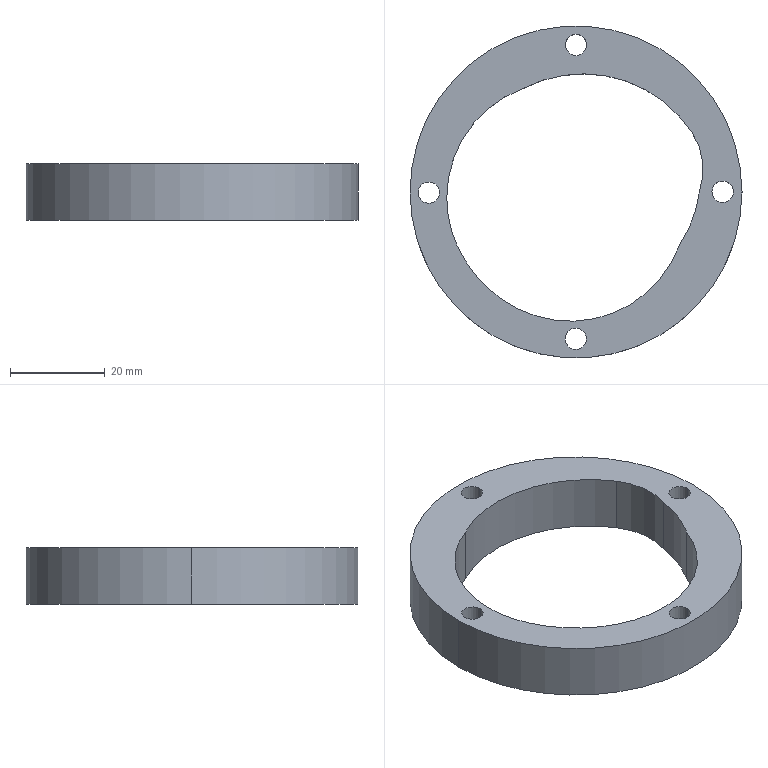Part | SolidWorks | features Extrusion 1, ICE 1 | 1 solid | 19 faces | box 70 x 70 x 12 mm | volume 19285 mm3 | cylinder 17 | plane 2 | commonest cylinder face diameters 4.5 x8 49 x3 55 x2 70 x2 28.257 x1 50.6 x1
STEP:
#1=CARTESIAN_POINT('',(28.668,0.04939,0.));
#2=VERTEX_POINT('',#1);
#3=CARTESIAN_POINT('',(33.168,0.04939,0.));
#4=VERTEX_POINT('',#3);
#5=CARTESIAN_POINT('',(30.918,0.04939,0.));
#6=DIRECTION('',(0.,0.,1.));
#7=DIRECTION('',(1.,0.,0.));
#8=AXIS2_PLACEMENT_3D('',#5,#6,#7);
#9=CIRCLE('',#8,2.25);
#10=EDGE_CURVE('',#2,#4,#9,.T.);
#11=ORIENTED_EDGE('',*,*,#10,.F.);
#12=CARTESIAN_POINT('',(28.668,0.04939,12.));
#13=VERTEX_POINT('',#12);
#14=CARTESIAN_POINT('',(28.668,0.04939,0.));
#15=DIRECTION('',(0.,0.,1.));
#16=VECTOR('',#15,1000.);
#17=LINE('',#14,#16);
#18=EDGE_CURVE('',#2,#13,#17,.T.);
#19=ORIENTED_EDGE('',*,*,#18,.T.);
#20=CARTESIAN_POINT('',(33.168,0.04939,12.));
#21=VERTEX_POINT('',#20);
#22=CARTESIAN_POINT('',(30.918,0.04939,12.));
#23=DIRECTION('',(0.,0.,1.));
#24=DIRECTION('',(1.,0.,0.));
#25=AXIS2_PLACEMENT_3D('',#22,#23,#24);
#26=CIRCLE('',#25,2.25);
#27=EDGE_CURVE('',#13,#21,#26,.T.);
#28=ORIENTED_EDGE('',*,*,#27,.T.);
#29=CARTESIAN_POINT('',(33.168,0.04939,0.));
#30=DIRECTION('',(0.,0.,1.));
#31=VECTOR('',#30,1000.);
#32=LINE('',#29,#31);
#33=EDGE_CURVE('',#4,#21,#32,.T.);
#34=ORIENTED_EDGE('',*,*,#33,.F.);
#35=EDGE_LOOP('',(#11,#19,#28,#34));
#36=FACE_OUTER_BOUND('',#35,.T.);
#37=CARTESIAN_POINT('',(30.918,0.04939,0.));
#38=DIRECTION('',(0.,0.,1.));
#39=DIRECTION('',(1.,0.,0.));
#40=AXIS2_PLACEMENT_3D('',#37,#38,#39);
#41=CYLINDRICAL_SURFACE('',#40,2.25);
#42=ADVANCED_FACE('',(#36),#41,.F.);
#43=CARTESIAN_POINT('',(-2.297,-30.979,0.));
#44=VERTEX_POINT('',#43);
#45=CARTESIAN_POINT('',(2.203,-30.979,0.));
#46=VERTEX_POINT('',#45);
#47=CARTESIAN_POINT('',(-0.04741,-30.979,0.));
#48=DIRECTION('',(0.,0.,1.));
#49=DIRECTION('',(1.,0.,0.));
#50=AXIS2_PLACEMENT_3D('',#47,#48,#49);
#51=CIRCLE('',#50,2.25);
#52=EDGE_CURVE('',#44,#46,#51,.T.);
#53=ORIENTED_EDGE('',*,*,#52,.F.);
#54=CARTESIAN_POINT('',(-2.297,-30.979,12.));
#55=VERTEX_POINT('',#54);
#56=CARTESIAN_POINT('',(-2.297,-30.979,0.));
#57=DIRECTION('',(0.,0.,1.));
#58=VECTOR('',#57,1000.);
#59=LINE('',#56,#58);
#60=EDGE_CURVE('',#44,#55,#59,.T.);
#61=ORIENTED_EDGE('',*,*,#60,.T.);
#62=CARTESIAN_POINT('',(2.203,-30.979,12.));
#63=VERTEX_POINT('',#62);
#64=CARTESIAN_POINT('',(-0.04741,-30.979,12.));
#65=DIRECTION('',(0.,0.,1.));
#66=DIRECTION('',(1.,0.,0.));
#67=AXIS2_PLACEMENT_3D('',#64,#65,#66);
#68=CIRCLE('',#67,2.25);
#69=EDGE_CURVE('',#55,#63,#68,.T.);
#70=ORIENTED_EDGE('',*,*,#69,.T.);
#71=CARTESIAN_POINT('',(2.203,-30.979,0.));
#72=DIRECTION('',(0.,0.,1.));
#73=VECTOR('',#72,1000.);
#74=LINE('',#71,#73);
#75=EDGE_CURVE('',#46,#63,#74,.T.);
#76=ORIENTED_EDGE('',*,*,#75,.F.);
#77=EDGE_LOOP('',(#53,#61,#70,#76));
#78=FACE_OUTER_BOUND('',#77,.T.);
#79=CARTESIAN_POINT('',(-0.04741,-30.979,0.));
#80=DIRECTION('',(0.,0.,1.));
#81=DIRECTION('',(1.,0.,0.));
#82=AXIS2_PLACEMENT_3D('',#79,#80,#81);
#83=CYLINDRICAL_SURFACE('',#82,2.25);
#84=ADVANCED_FACE('',(#78),#83,.F.);
#85=CARTESIAN_POINT('',(-33.267,-0.1482,0.));
#86=VERTEX_POINT('',#85);
#87=CARTESIAN_POINT('',(-28.767,-0.1482,0.));
#88=VERTEX_POINT('',#87);
#89=CARTESIAN_POINT('',(-31.017,-0.1482,0.));
#90=DIRECTION('',(0.,0.,1.));
#91=DIRECTION('',(1.,0.,0.));
#92=AXIS2_PLACEMENT_3D('',#89,#90,#91);
#93=CIRCLE('',#92,2.25);
#94=EDGE_CURVE('',#86,#88,#93,.T.);
#95=ORIENTED_EDGE('',*,*,#94,.F.);
#96=CARTESIAN_POINT('',(-33.267,-0.1482,12.));
#97=VERTEX_POINT('',#96);
#98=CARTESIAN_POINT('',(-33.267,-0.1482,0.));
#99=DIRECTION('',(0.,0.,1.));
#100=VECTOR('',#99,1000.);
#101=LINE('',#98,#100);
#102=EDGE_CURVE('',#86,#97,#101,.T.);
#103=ORIENTED_EDGE('',*,*,#102,.T.);
#104=CARTESIAN_POINT('',(-28.767,-0.1482,12.));
#105=VERTEX_POINT('',#104);
#106=CARTESIAN_POINT('',(-31.017,-0.1482,12.));
#107=DIRECTION('',(0.,0.,1.));
#108=DIRECTION('',(1.,0.,0.));
#109=AXIS2_PLACEMENT_3D('',#106,#107,#108);
#110=CIRCLE('',#109,2.25);
#111=EDGE_CURVE('',#97,#105,#110,.T.);
#112=ORIENTED_EDGE('',*,*,#111,.T.);
#113=CARTESIAN_POINT('',(-28.767,-0.1482,0.));
#114=DIRECTION('',(0.,0.,1.));
#115=VECTOR('',#114,1000.);
#116=LINE('',#113,#115);
#117=EDGE_CURVE('',#88,#105,#116,.T.);
#118=ORIENTED_EDGE('',*,*,#117,.F.);
#119=EDGE_LOOP('',(#95,#103,#112,#118));
#120=FACE_OUTER_BOUND('',#119,.T.);
#121=CARTESIAN_POINT('',(-31.017,-0.1482,0.));
#122=DIRECTION('',(0.,0.,1.));
#123=DIRECTION('',(1.,0.,0.));
#124=AXIS2_PLACEMENT_3D('',#121,#122,#123);
#125=CYLINDRICAL_SURFACE('',#124,2.25);
#126=ADVANCED_FACE('',(#120),#125,.F.);
#127=CARTESIAN_POINT('',(-2.25,31.,0.));
#128=VERTEX_POINT('',#127);
#129=CARTESIAN_POINT('',(2.25,31.,0.));
#130=VERTEX_POINT('',#129);
#131=CARTESIAN_POINT('',(0.,31.,0.));
#132=DIRECTION('',(0.,0.,1.));
#133=DIRECTION('',(1.,0.,0.));
#134=AXIS2_PLACEMENT_3D('',#131,#132,#133);
#135=CIRCLE('',#134,2.25);
#136=EDGE_CURVE('',#128,#130,#135,.T.);
#137=ORIENTED_EDGE('',*,*,#136,.F.);
#138=CARTESIAN_POINT('',(-2.25,31.,12.));
#139=VERTEX_POINT('',#138);
#140=CARTESIAN_POINT('',(-2.25,31.,0.));
#141=DIRECTION('',(0.,0.,1.));
#142=VECTOR('',#141,1000.);
#143=LINE('',#140,#142);
#144=EDGE_CURVE('',#128,#139,#143,.T.);
#145=ORIENTED_EDGE('',*,*,#144,.T.);
#146=CARTESIAN_POINT('',(2.25,31.,12.));
#147=VERTEX_POINT('',#146);
#148=CARTESIAN_POINT('',(0.,31.,12.));
#149=DIRECTION('',(0.,0.,1.));
#150=DIRECTION('',(1.,0.,0.));
#151=AXIS2_PLACEMENT_3D('',#148,#149,#150);
#152=CIRCLE('',#151,2.25);
#153=EDGE_CURVE('',#139,#147,#152,.T.);
#154=ORIENTED_EDGE('',*,*,#153,.T.);
#155=CARTESIAN_POINT('',(2.25,31.,0.));
#156=DIRECTION('',(0.,0.,1.));
#157=VECTOR('',#156,1000.);
#158=LINE('',#155,#157);
#159=EDGE_CURVE('',#130,#147,#158,.T.);
#160=ORIENTED_EDGE('',*,*,#159,.F.);
#161=EDGE_LOOP('',(#137,#145,#154,#160));
#162=FACE_OUTER_BOUND('',#161,.T.);
#163=CARTESIAN_POINT('',(0.,31.,0.));
#164=DIRECTION('',(0.,0.,1.));
#165=DIRECTION('',(1.,0.,0.));
#166=AXIS2_PLACEMENT_3D('',#163,#164,#165);
#167=CYLINDRICAL_SURFACE('',#166,2.25);
#168=ADVANCED_FACE('',(#162),#167,.F.);
#169=CARTESIAN_POINT('',(35.,0.,12.));
#170=VERTEX_POINT('',#169);
#171=CARTESIAN_POINT('',(-35.,0.,12.));
#172=VERTEX_POINT('',#171);
#173=CARTESIAN_POINT('',(0.,0.,12.));
#174=DIRECTION('',(0.,0.,1.));
#175=DIRECTION('',(1.,0.,0.));
#176=AXIS2_PLACEMENT_3D('',#173,#174,#175);
#177=CIRCLE('',#176,35.);
#178=EDGE_CURVE('',#170,#172,#177,.T.);
#179=ORIENTED_EDGE('',*,*,#178,.F.);
#180=CARTESIAN_POINT('',(35.,0.,0.));
#181=VERTEX_POINT('',#180);
#182=CARTESIAN_POINT('',(35.,0.,12.));
#183=DIRECTION('',(0.,0.,-1.));
#184=VECTOR('',#183,1000.);
#185=LINE('',#182,#184);
#186=EDGE_CURVE('',#170,#181,#185,.T.);
#187=ORIENTED_EDGE('',*,*,#186,.T.);
#188=CARTESIAN_POINT('',(-35.,0.,0.));
#189=VERTEX_POINT('',#188);
#190=CARTESIAN_POINT('',(0.,0.,0.));
#191=DIRECTION('',(0.,0.,1.));
#192=DIRECTION('',(1.,0.,0.));
#193=AXIS2_PLACEMENT_3D('',#190,#191,#192);
#194=CIRCLE('',#193,35.);
#195=EDGE_CURVE('',#181,#189,#194,.T.);
#196=ORIENTED_EDGE('',*,*,#195,.T.);
#197=CARTESIAN_POINT('',(-35.,0.,12.));
#198=DIRECTION('',(0.,0.,-1.));
#199=VECTOR('',#198,1000.);
#200=LINE('',#197,#199);
#201=EDGE_CURVE('',#172,#189,#200,.T.);
#202=ORIENTED_EDGE('',*,*,#201,.F.);
#203=EDGE_LOOP('',(#179,#187,#196,#202));
#204=FACE_OUTER_BOUND('',#203,.T.);
#205=CARTESIAN_POINT('',(0.,0.,12.));
#206=DIRECTION('',(0.,0.,-1.));
#207=DIRECTION('',(-1.,0.,0.));
#208=AXIS2_PLACEMENT_3D('',#205,#206,#207);
#209=CYLINDRICAL_SURFACE('',#208,35.);
#210=ADVANCED_FACE('',(#204),#209,.T.);
#211=CARTESIAN_POINT('',(-27.251,-1.196,12.));
#212=VERTEX_POINT('',#211);
#213=CARTESIAN_POINT('',(-11.123,21.83,12.));
#214=VERTEX_POINT('',#213);
#215=CARTESIAN_POINT('',(-2.751,-1.196,12.));
#216=DIRECTION('',(0.,0.,-1.));
#217=DIRECTION('',(1.,0.,0.));
#218=AXIS2_PLACEMENT_3D('',#215,#216,#217);
#219=CIRCLE('',#218,24.5);
#220=EDGE_CURVE('',#212,#214,#219,.T.);
#221=ORIENTED_EDGE('',*,*,#220,.F.);
#222=CARTESIAN_POINT('',(-27.251,-1.196,0.));
#223=VERTEX_POINT('',#222);
#224=CARTESIAN_POINT('',(-27.251,-1.196,12.));
#225=DIRECTION('',(0.,0.,-1.));
#226=VECTOR('',#225,1000.);
#227=LINE('',#224,#226);
#228=EDGE_CURVE('',#212,#223,#227,.T.);
#229=ORIENTED_EDGE('',*,*,#228,.T.);
#230=CARTESIAN_POINT('',(-11.123,21.83,0.));
#231=VERTEX_POINT('',#230);
#232=CARTESIAN_POINT('',(-2.751,-1.196,0.));
#233=DIRECTION('',(0.,0.,-1.));
#234=DIRECTION('',(1.,0.,0.));
#235=AXIS2_PLACEMENT_3D('',#232,#233,#234);
#236=CIRCLE('',#235,24.5);
#237=EDGE_CURVE('',#223,#231,#236,.T.);
#238=ORIENTED_EDGE('',*,*,#237,.T.);
#239=CARTESIAN_POINT('',(-11.123,21.83,12.));
#240=DIRECTION('',(0.,0.,-1.));
#241=VECTOR('',#240,1000.);
#242=LINE('',#239,#241);
#243=EDGE_CURVE('',#214,#231,#242,.T.);
#244=ORIENTED_EDGE('',*,*,#243,.F.);
#245=EDGE_LOOP('',(#221,#229,#238,#244));
#246=FACE_OUTER_BOUND('',#245,.T.);
#247=CARTESIAN_POINT('',(-2.751,-1.196,12.));
#248=DIRECTION('',(0.,0.,-1.));
#249=DIRECTION('',(-1.,0.,0.));
#250=AXIS2_PLACEMENT_3D('',#247,#248,#249);
#251=CYLINDRICAL_SURFACE('',#250,24.5);
#252=ADVANCED_FACE('',(#246),#251,.F.);
#253=CARTESIAN_POINT('',(-12.485,-24.503,0.));
#254=VERTEX_POINT('',#253);
#255=CARTESIAN_POINT('',(21.83,-11.123,0.));
#256=VERTEX_POINT('',#255);
#257=CARTESIAN_POINT('',(-1.198,-2.757,0.));
#258=DIRECTION('',(0.,0.,1.));
#259=DIRECTION('',(1.,0.,0.));
#260=AXIS2_PLACEMENT_3D('',#257,#258,#259);
#261=CIRCLE('',#260,24.5);
#262=EDGE_CURVE('',#254,#256,#261,.T.);
#263=ORIENTED_EDGE('',*,*,#262,.F.);
#264=CARTESIAN_POINT('',(-12.485,-24.503,12.));
#265=VERTEX_POINT('',#264);
#266=CARTESIAN_POINT('',(-12.485,-24.503,12.));
#267=DIRECTION('',(0.,0.,-1.));
#268=VECTOR('',#267,1000.);
#269=LINE('',#266,#268);
#270=EDGE_CURVE('',#265,#254,#269,.T.);
#271=ORIENTED_EDGE('',*,*,#270,.F.);
#272=CARTESIAN_POINT('',(21.83,-11.123,12.));
#273=VERTEX_POINT('',#272);
#274=CARTESIAN_POINT('',(-1.198,-2.757,12.));
#275=DIRECTION('',(0.,0.,1.));
#276=DIRECTION('',(1.,0.,0.));
#277=AXIS2_PLACEMENT_3D('',#274,#275,#276);
#278=CIRCLE('',#277,24.5);
#279=EDGE_CURVE('',#265,#273,#278,.T.);
#280=ORIENTED_EDGE('',*,*,#279,.T.);
#281=CARTESIAN_POINT('',(21.83,-11.123,12.));
#282=DIRECTION('',(0.,0.,-1.));
#283=VECTOR('',#282,1000.);
#284=LINE('',#281,#283);
#285=EDGE_CURVE('',#273,#256,#284,.T.);
#286=ORIENTED_EDGE('',*,*,#285,.T.);
#287=EDGE_LOOP('',(#263,#271,#280,#286));
#288=FACE_OUTER_BOUND('',#287,.T.);
#289=CARTESIAN_POINT('',(-1.198,-2.757,12.));
#290=DIRECTION('',(0.,0.,-1.));
#291=DIRECTION('',(-1.,0.,0.));
#292=AXIS2_PLACEMENT_3D('',#289,#290,#291);
#293=CYLINDRICAL_SURFACE('',#292,24.5);
#294=ADVANCED_FACE('',(#288),#293,.F.);
#295=CARTESIAN_POINT('',(-25.221,-10.961,0.));
#296=VERTEX_POINT('',#295);
#297=CARTESIAN_POINT('',(0.,0.,0.));
#298=DIRECTION('',(0.,0.,1.));
#299=DIRECTION('',(1.,0.,0.));
#300=AXIS2_PLACEMENT_3D('',#297,#298,#299);
#301=CIRCLE('',#300,27.5);
#302=EDGE_CURVE('',#296,#254,#301,.T.);
#303=ORIENTED_EDGE('',*,*,#302,.F.);
#304=CARTESIAN_POINT('',(-25.221,-10.961,12.));
#305=VERTEX_POINT('',#304);
#306=CARTESIAN_POINT('',(-25.221,-10.961,12.));
#307=DIRECTION('',(0.,0.,-1.));
#308=VECTOR('',#307,1000.);
#309=LINE('',#306,#308);
#310=EDGE_CURVE('',#305,#296,#309,.T.);
#311=ORIENTED_EDGE('',*,*,#310,.F.);
#312=CARTESIAN_POINT('',(0.,0.,12.));
#313=DIRECTION('',(0.,0.,1.));
#314=DIRECTION('',(1.,0.,0.));
#315=AXIS2_PLACEMENT_3D('',#312,#313,#314);
#316=CIRCLE('',#315,27.5);
#317=EDGE_CURVE('',#305,#265,#316,.T.);
#318=ORIENTED_EDGE('',*,*,#317,.T.);
#319=ORIENTED_EDGE('',*,*,#270,.T.);
#320=EDGE_LOOP('',(#303,#311,#318,#319));
#321=FACE_OUTER_BOUND('',#320,.T.);
#322=CARTESIAN_POINT('',(0.,0.,12.));
#323=DIRECTION('',(0.,0.,-1.));
#324=DIRECTION('',(-1.,0.,0.));
#325=AXIS2_PLACEMENT_3D('',#322,#323,#324);
#326=CYLINDRICAL_SURFACE('',#325,27.5);
#327=ADVANCED_FACE('',(#321),#326,.F.);
#328=ORIENTED_EDGE('',*,*,#228,.F.);
#329=CARTESIAN_POINT('',(-2.751,-1.196,12.));
#330=DIRECTION('',(0.,0.,-1.));
#331=DIRECTION('',(1.,0.,0.));
#332=AXIS2_PLACEMENT_3D('',#329,#330,#331);
#333=CIRCLE('',#332,24.5);
#334=EDGE_CURVE('',#305,#212,#333,.T.);
#335=ORIENTED_EDGE('',*,*,#334,.F.);
#336=ORIENTED_EDGE('',*,*,#310,.T.);
#337=CARTESIAN_POINT('',(-2.751,-1.196,0.));
#338=DIRECTION('',(0.,0.,-1.));
#339=DIRECTION('',(1.,0.,0.));
#340=AXIS2_PLACEMENT_3D('',#337,#338,#339);
#341=CIRCLE('',#340,24.5);
#342=EDGE_CURVE('',#296,#223,#341,.T.);
#343=ORIENTED_EDGE('',*,*,#342,.T.);
#344=EDGE_LOOP('',(#328,#335,#336,#343));
#345=FACE_OUTER_BOUND('',#344,.T.);
#346=CARTESIAN_POINT('',(-2.751,-1.196,12.));
#347=DIRECTION('',(0.,0.,-1.));
#348=DIRECTION('',(-1.,0.,0.));
#349=AXIS2_PLACEMENT_3D('',#346,#347,#348);
#350=CYLINDRICAL_SURFACE('',#349,24.5);
#351=ADVANCED_FACE('',(#345),#350,.F.);
#352=CARTESIAN_POINT('',(24.503,12.485,0.));
#353=VERTEX_POINT('',#352);
#354=CARTESIAN_POINT('',(1.508,-2.598,0.));
#355=DIRECTION('',(0.,0.,-1.));
#356=DIRECTION('',(1.,0.,0.));
#357=AXIS2_PLACEMENT_3D('',#354,#355,#356);
#358=CIRCLE('',#357,27.5);
#359=EDGE_CURVE('',#231,#353,#358,.T.);
#360=ORIENTED_EDGE('',*,*,#359,.T.);
#361=CARTESIAN_POINT('',(24.503,12.485,12.));
#362=VERTEX_POINT('',#361);
#363=CARTESIAN_POINT('',(24.503,12.485,12.));
#364=DIRECTION('',(0.,0.,-1.));
#365=VECTOR('',#364,1000.);
#366=LINE('',#363,#365);
#367=EDGE_CURVE('',#362,#353,#366,.T.);
#368=ORIENTED_EDGE('',*,*,#367,.F.);
#369=CARTESIAN_POINT('',(1.508,-2.598,12.));
#370=DIRECTION('',(0.,0.,-1.));
#371=DIRECTION('',(1.,0.,0.));
#372=AXIS2_PLACEMENT_3D('',#369,#370,#371);
#373=CIRCLE('',#372,27.5);
#374=EDGE_CURVE('',#214,#362,#373,.T.);
#375=ORIENTED_EDGE('',*,*,#374,.F.);
#376=ORIENTED_EDGE('',*,*,#243,.T.);
#377=EDGE_LOOP('',(#360,#368,#375,#376));
#378=FACE_OUTER_BOUND('',#377,.T.);
#379=CARTESIAN_POINT('',(1.508,-2.598,12.));
#380=DIRECTION('',(0.,0.,-1.));
#381=DIRECTION('',(-1.,0.,0.));
#382=AXIS2_PLACEMENT_3D('',#379,#380,#381);
#383=CYLINDRICAL_SURFACE('',#382,27.5);
#384=ADVANCED_FACE('',(#378),#383,.F.);
#385=CARTESIAN_POINT('',(26.,0.,0.));
#386=VERTEX_POINT('',#385);
#387=CARTESIAN_POINT('',(12.689,4.736,0.));
#388=DIRECTION('',(0.,0.,-1.));
#389=DIRECTION('',(1.,0.,0.));
#390=AXIS2_PLACEMENT_3D('',#387,#388,#389);
#391=CIRCLE('',#390,14.129);
#392=EDGE_CURVE('',#353,#386,#391,.T.);
#393=ORIENTED_EDGE('',*,*,#392,.T.);
#394=CARTESIAN_POINT('',(26.,0.,12.));
#395=VERTEX_POINT('',#394);
#396=CARTESIAN_POINT('',(26.,0.,12.));
#397=DIRECTION('',(0.,0.,-1.));
#398=VECTOR('',#397,1000.);
#399=LINE('',#396,#398);
#400=EDGE_CURVE('',#395,#386,#399,.T.);
#401=ORIENTED_EDGE('',*,*,#400,.F.);
#402=CARTESIAN_POINT('',(12.689,4.736,12.));
#403=DIRECTION('',(0.,0.,-1.));
#404=DIRECTION('',(1.,0.,0.));
#405=AXIS2_PLACEMENT_3D('',#402,#403,#404);
#406=CIRCLE('',#405,14.129);
#407=EDGE_CURVE('',#362,#395,#406,.T.);
#408=ORIENTED_EDGE('',*,*,#407,.F.);
#409=ORIENTED_EDGE('',*,*,#367,.T.);
#410=EDGE_LOOP('',(#393,#401,#408,#409));
#411=FACE_OUTER_BOUND('',#410,.T.);
#412=CARTESIAN_POINT('',(12.689,4.736,12.));
#413=DIRECTION('',(0.,0.,-1.));
#414=DIRECTION('',(-1.,0.,0.));
#415=AXIS2_PLACEMENT_3D('',#412,#413,#414);
#416=CYLINDRICAL_SURFACE('',#415,14.129);
#417=ADVANCED_FACE('',(#411),#416,.F.);
#418=CARTESIAN_POINT('',(0.8873,3.073,0.));
#419=DIRECTION('',(0.,0.,-1.));
#420=DIRECTION('',(1.,0.,0.));
#421=AXIS2_PLACEMENT_3D('',#418,#419,#420);
#422=CIRCLE('',#421,25.3);
#423=EDGE_CURVE('',#386,#256,#422,.T.);
#424=ORIENTED_EDGE('',*,*,#423,.T.);
#425=ORIENTED_EDGE('',*,*,#285,.F.);
#426=CARTESIAN_POINT('',(0.8873,3.073,12.));
#427=DIRECTION('',(0.,0.,-1.));
#428=DIRECTION('',(1.,0.,0.));
#429=AXIS2_PLACEMENT_3D('',#426,#427,#428);
#430=CIRCLE('',#429,25.3);
#431=EDGE_CURVE('',#395,#273,#430,.T.);
#432=ORIENTED_EDGE('',*,*,#431,.F.);
#433=ORIENTED_EDGE('',*,*,#400,.T.);
#434=EDGE_LOOP('',(#424,#425,#432,#433));
#435=FACE_OUTER_BOUND('',#434,.T.);
#436=CARTESIAN_POINT('',(0.8873,3.073,12.));
#437=DIRECTION('',(0.,0.,-1.));
#438=DIRECTION('',(-1.,0.,0.));
#439=AXIS2_PLACEMENT_3D('',#436,#437,#438);
#440=CYLINDRICAL_SURFACE('',#439,25.3);
#441=ADVANCED_FACE('',(#435),#440,.F.);
#442=ORIENTED_EDGE('',*,*,#186,.F.);
#443=CARTESIAN_POINT('',(0.,0.,12.));
#444=DIRECTION('',(0.,0.,1.));
#445=DIRECTION('',(1.,0.,0.));
#446=AXIS2_PLACEMENT_3D('',#443,#444,#445);
#447=CIRCLE('',#446,35.);
#448=EDGE_CURVE('',#172,#170,#447,.T.);
#449=ORIENTED_EDGE('',*,*,#448,.F.);
#450=ORIENTED_EDGE('',*,*,#201,.T.);
#451=CARTESIAN_POINT('',(0.,0.,0.));
#452=DIRECTION('',(0.,0.,1.));
#453=DIRECTION('',(1.,0.,0.));
#454=AXIS2_PLACEMENT_3D('',#451,#452,#453);
#455=CIRCLE('',#454,35.);
#456=EDGE_CURVE('',#189,#181,#455,.T.);
#457=ORIENTED_EDGE('',*,*,#456,.T.);
#458=EDGE_LOOP('',(#442,#449,#450,#457));
#459=FACE_OUTER_BOUND('',#458,.T.);
#460=CARTESIAN_POINT('',(0.,0.,12.));
#461=DIRECTION('',(0.,0.,-1.));
#462=DIRECTION('',(-1.,0.,0.));
#463=AXIS2_PLACEMENT_3D('',#460,#461,#462);
#464=CYLINDRICAL_SURFACE('',#463,35.);
#465=ADVANCED_FACE('',(#459),#464,.T.);
#466=CARTESIAN_POINT('',(30.918,0.04939,12.));
#467=DIRECTION('',(0.,0.,1.));
#468=DIRECTION('',(1.,0.,0.));
#469=AXIS2_PLACEMENT_3D('',#466,#467,#468);
#470=CIRCLE('',#469,2.25);
#471=EDGE_CURVE('',#21,#13,#470,.T.);
#472=ORIENTED_EDGE('',*,*,#471,.F.);
#473=ORIENTED_EDGE('',*,*,#27,.F.);
#474=EDGE_LOOP('',(#472,#473));
#475=FACE_BOUND('',#474,.T.);
#476=CARTESIAN_POINT('',(-0.04741,-30.979,12.));
#477=DIRECTION('',(0.,0.,1.));
#478=DIRECTION('',(1.,0.,0.));
#479=AXIS2_PLACEMENT_3D('',#476,#477,#478);
#480=CIRCLE('',#479,2.25);
#481=EDGE_CURVE('',#63,#55,#480,.T.);
#482=ORIENTED_EDGE('',*,*,#481,.F.);
#483=ORIENTED_EDGE('',*,*,#69,.F.);
#484=EDGE_LOOP('',(#482,#483));
#485=FACE_BOUND('',#484,.T.);
#486=CARTESIAN_POINT('',(-31.017,-0.1482,12.));
#487=DIRECTION('',(0.,0.,1.));
#488=DIRECTION('',(1.,0.,0.));
#489=AXIS2_PLACEMENT_3D('',#486,#487,#488);
#490=CIRCLE('',#489,2.25);
#491=EDGE_CURVE('',#105,#97,#490,.T.);
#492=ORIENTED_EDGE('',*,*,#491,.F.);
#493=ORIENTED_EDGE('',*,*,#111,.F.);
#494=EDGE_LOOP('',(#492,#493));
#495=FACE_BOUND('',#494,.T.);
#496=CARTESIAN_POINT('',(0.,31.,12.));
#497=DIRECTION('',(0.,0.,1.));
#498=DIRECTION('',(1.,0.,0.));
#499=AXIS2_PLACEMENT_3D('',#496,#497,#498);
#500=CIRCLE('',#499,2.25);
#501=EDGE_CURVE('',#147,#139,#500,.T.);
#502=ORIENTED_EDGE('',*,*,#501,.F.);
#503=ORIENTED_EDGE('',*,*,#153,.F.);
#504=EDGE_LOOP('',(#502,#503));
#505=FACE_BOUND('',#504,.T.);
#506=ORIENTED_EDGE('',*,*,#279,.F.);
#507=ORIENTED_EDGE('',*,*,#317,.F.);
#508=ORIENTED_EDGE('',*,*,#334,.T.);
#509=ORIENTED_EDGE('',*,*,#220,.T.);
#510=ORIENTED_EDGE('',*,*,#374,.T.);
#511=ORIENTED_EDGE('',*,*,#407,.T.);
#512=ORIENTED_EDGE('',*,*,#431,.T.);
#513=EDGE_LOOP('',(#506,#507,#508,#509,#510,#511,#512));
#514=FACE_BOUND('',#513,.T.);
#515=ORIENTED_EDGE('',*,*,#448,.T.);
#516=ORIENTED_EDGE('',*,*,#178,.T.);
#517=EDGE_LOOP('',(#515,#516));
#518=FACE_OUTER_BOUND('',#517,.T.);
#519=CARTESIAN_POINT('',(0.,0.,12.));
#520=DIRECTION('',(0.,0.,1.));
#521=DIRECTION('',(1.,0.,0.));
#522=AXIS2_PLACEMENT_3D('',#519,#520,#521);
#523=PLANE('',#522);
#524=ADVANCED_FACE('',(#475,#485,#495,#505,#514,#518),#523,.T.);
#525=CARTESIAN_POINT('',(30.918,0.04939,0.));
#526=DIRECTION('',(0.,0.,1.));
#527=DIRECTION('',(1.,0.,0.));
#528=AXIS2_PLACEMENT_3D('',#525,#526,#527);
#529=CIRCLE('',#528,2.25);
#530=EDGE_CURVE('',#4,#2,#529,.T.);
#531=ORIENTED_EDGE('',*,*,#530,.T.);
#532=ORIENTED_EDGE('',*,*,#10,.T.);
#533=EDGE_LOOP('',(#531,#532));
#534=FACE_BOUND('',#533,.T.);
#535=CARTESIAN_POINT('',(-0.04741,-30.979,0.));
#536=DIRECTION('',(0.,0.,1.));
#537=DIRECTION('',(1.,0.,0.));
#538=AXIS2_PLACEMENT_3D('',#535,#536,#537);
#539=CIRCLE('',#538,2.25);
#540=EDGE_CURVE('',#46,#44,#539,.T.);
#541=ORIENTED_EDGE('',*,*,#540,.T.);
#542=ORIENTED_EDGE('',*,*,#52,.T.);
#543=EDGE_LOOP('',(#541,#542));
#544=FACE_BOUND('',#543,.T.);
#545=CARTESIAN_POINT('',(-31.017,-0.1482,0.));
#546=DIRECTION('',(0.,0.,1.));
#547=DIRECTION('',(1.,0.,0.));
#548=AXIS2_PLACEMENT_3D('',#545,#546,#547);
#549=CIRCLE('',#548,2.25);
#550=EDGE_CURVE('',#88,#86,#549,.T.);
#551=ORIENTED_EDGE('',*,*,#550,.T.);
#552=ORIENTED_EDGE('',*,*,#94,.T.);
#553=EDGE_LOOP('',(#551,#552));
#554=FACE_BOUND('',#553,.T.);
#555=CARTESIAN_POINT('',(0.,31.,0.));
#556=DIRECTION('',(0.,0.,1.));
#557=DIRECTION('',(1.,0.,0.));
#558=AXIS2_PLACEMENT_3D('',#555,#556,#557);
#559=CIRCLE('',#558,2.25);
#560=EDGE_CURVE('',#130,#128,#559,.T.);
#561=ORIENTED_EDGE('',*,*,#560,.T.);
#562=ORIENTED_EDGE('',*,*,#136,.T.);
#563=EDGE_LOOP('',(#561,#562));
#564=FACE_BOUND('',#563,.T.);
#565=ORIENTED_EDGE('',*,*,#262,.T.);
#566=ORIENTED_EDGE('',*,*,#423,.F.);
#567=ORIENTED_EDGE('',*,*,#392,.F.);
#568=ORIENTED_EDGE('',*,*,#359,.F.);
#569=ORIENTED_EDGE('',*,*,#237,.F.);
#570=ORIENTED_EDGE('',*,*,#342,.F.);
#571=ORIENTED_EDGE('',*,*,#302,.T.);
#572=EDGE_LOOP('',(#565,#566,#567,#568,#569,#570,#571));
#573=FACE_BOUND('',#572,.T.);
#574=ORIENTED_EDGE('',*,*,#456,.F.);
#575=ORIENTED_EDGE('',*,*,#195,.F.);
#576=EDGE_LOOP('',(#574,#575));
#577=FACE_OUTER_BOUND('',#576,.T.);
#578=CARTESIAN_POINT('',(0.,0.,0.));
#579=DIRECTION('',(0.,0.,1.));
#580=DIRECTION('',(1.,0.,0.));
#581=AXIS2_PLACEMENT_3D('',#578,#579,#580);
#582=PLANE('',#581);
#583=ADVANCED_FACE('',(#534,#544,#554,#564,#573,#577),#582,.F.);
#584=ORIENTED_EDGE('',*,*,#144,.F.);
#585=ORIENTED_EDGE('',*,*,#560,.F.);
#586=ORIENTED_EDGE('',*,*,#159,.T.);
#587=ORIENTED_EDGE('',*,*,#501,.T.);
#588=EDGE_LOOP('',(#584,#585,#586,#587));
#589=FACE_OUTER_BOUND('',#588,.T.);
#590=CARTESIAN_POINT('',(0.,31.,0.));
#591=DIRECTION('',(0.,0.,1.));
#592=DIRECTION('',(1.,0.,0.));
#593=AXIS2_PLACEMENT_3D('',#590,#591,#592);
#594=CYLINDRICAL_SURFACE('',#593,2.25);
#595=ADVANCED_FACE('',(#589),#594,.F.);
#596=ORIENTED_EDGE('',*,*,#102,.F.);
#597=ORIENTED_EDGE('',*,*,#550,.F.);
#598=ORIENTED_EDGE('',*,*,#117,.T.);
#599=ORIENTED_EDGE('',*,*,#491,.T.);
#600=EDGE_LOOP('',(#596,#597,#598,#599));
#601=FACE_OUTER_BOUND('',#600,.T.);
#602=CARTESIAN_POINT('',(-31.017,-0.1482,0.));
#603=DIRECTION('',(0.,0.,1.));
#604=DIRECTION('',(1.,0.,0.));
#605=AXIS2_PLACEMENT_3D('',#602,#603,#604);
#606=CYLINDRICAL_SURFACE('',#605,2.25);
#607=ADVANCED_FACE('',(#601),#606,.F.);
#608=ORIENTED_EDGE('',*,*,#60,.F.);
#609=ORIENTED_EDGE('',*,*,#540,.F.);
#610=ORIENTED_EDGE('',*,*,#75,.T.);
#611=ORIENTED_EDGE('',*,*,#481,.T.);
#612=EDGE_LOOP('',(#608,#609,#610,#611));
#613=FACE_OUTER_BOUND('',#612,.T.);
#614=CARTESIAN_POINT('',(-0.04741,-30.979,0.));
#615=DIRECTION('',(0.,0.,1.));
#616=DIRECTION('',(1.,0.,0.));
#617=AXIS2_PLACEMENT_3D('',#614,#615,#616);
#618=CYLINDRICAL_SURFACE('',#617,2.25);
#619=ADVANCED_FACE('',(#613),#618,.F.);
#620=ORIENTED_EDGE('',*,*,#18,.F.);
#621=ORIENTED_EDGE('',*,*,#530,.F.);
#622=ORIENTED_EDGE('',*,*,#33,.T.);
#623=ORIENTED_EDGE('',*,*,#471,.T.);
#624=EDGE_LOOP('',(#620,#621,#622,#623));
#625=FACE_OUTER_BOUND('',#624,.T.);
#626=CARTESIAN_POINT('',(30.918,0.04939,0.));
#627=DIRECTION('',(0.,0.,1.));
#628=DIRECTION('',(1.,0.,0.));
#629=AXIS2_PLACEMENT_3D('',#626,#627,#628);
#630=CYLINDRICAL_SURFACE('',#629,2.25);
#631=ADVANCED_FACE('',(#625),#630,.F.);
#632=CLOSED_SHELL('',(#42,#84,#126,#168,#210,#252,#294,#327,#351,#384,#417,#441,#465,#524,#583,#595,#607,#619,#631));
#633=MANIFOLD_SOLID_BREP('',#632);
#634=CARTESIAN_POINT('',(0.,0.,0.));
#635=DIRECTION('',(0.,0.,1.));
#636=DIRECTION('',(1.,0.,0.));
#637=AXIS2_PLACEMENT_3D('',#634,#635,#636);
#638=(LENGTH_UNIT()NAMED_UNIT(*)SI_UNIT(.MILLI.,.METRE.));
#639=UNCERTAINTY_MEASURE_WITH_UNIT(LENGTH_MEASURE(0.00001),#638,'','');
#640=(NAMED_UNIT(*)PLANE_ANGLE_UNIT()SI_UNIT($,.RADIAN.));
#641=(NAMED_UNIT(*)SI_UNIT($,.STERADIAN.)SOLID_ANGLE_UNIT());
#642=(GEOMETRIC_REPRESENTATION_CONTEXT(3)GLOBAL_UNCERTAINTY_ASSIGNED_CONTEXT((#639))GLOBAL_UNIT_ASSIGNED_CONTEXT((#638,#640,#641))REPRESENTATION_CONTEXT('',''));
#643=ADVANCED_BREP_SHAPE_REPRESENTATION('',(#633,#637),#642);